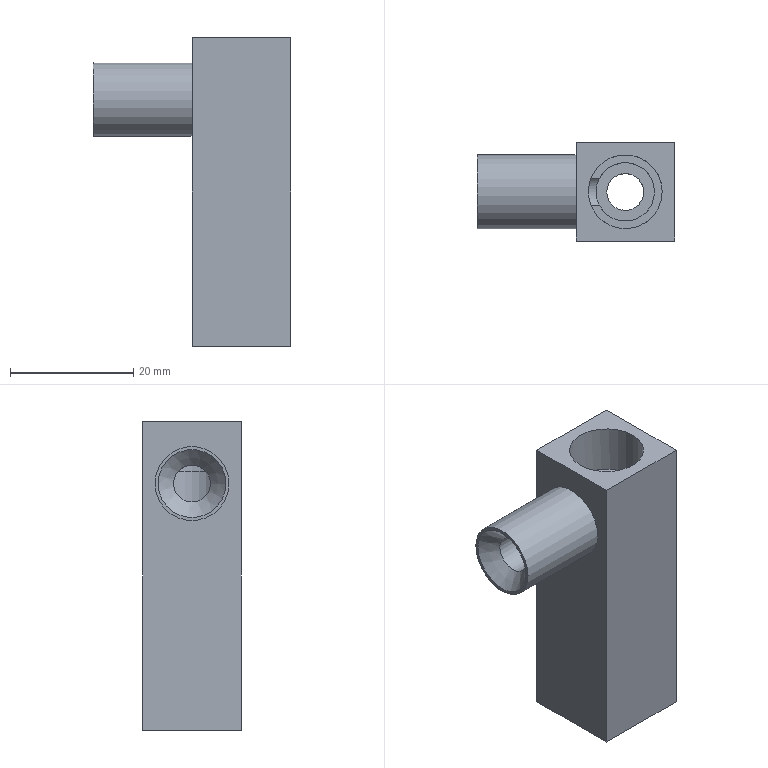Part | STEP file | 1-46.4 | 1 solid | 22 faces | box 32 x 16 x 50 mm | volume 9921 mm3 | plane 13 | cylinder 8 | cone 1 | commonest cylinder face diameters 12 x4 6 x2 9.5 x2